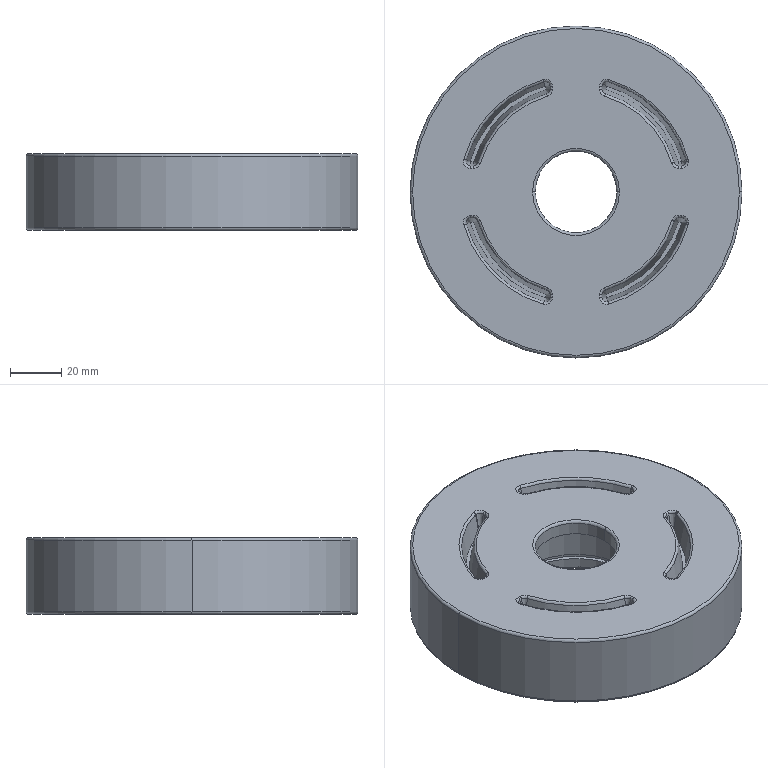Part | SolidWorks | features ICE 7, Fillet 2, CirPattern 1, Extrusion 1, MirrorPattern 1 | 1 solid | 183 faces | box 130 x 130 x 30 mm | volume 330858 mm3 | torus 60 | cone 56 | cylinder 34 | plane 33 | commonest cylinder face diameters 2 x16 3 x6 52 x4 32 x2 45 x2 55 x2